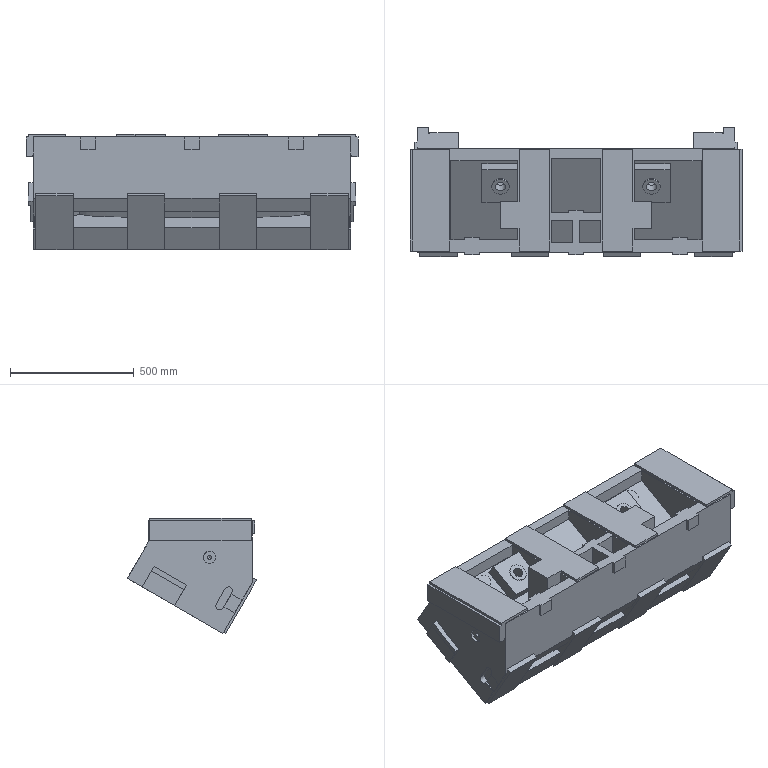Part | NX | features solid 2 | 1 solid | 344 faces | box 1340 x 521.542 x 464.641 mm | volume 120263051 mm3 | plane 304 | cylinder 32 | spline 6 | cone 2 | commonest cylinder face diameters 50 x10 55 x5 90 x5 32 x4 16 x2 40 x2